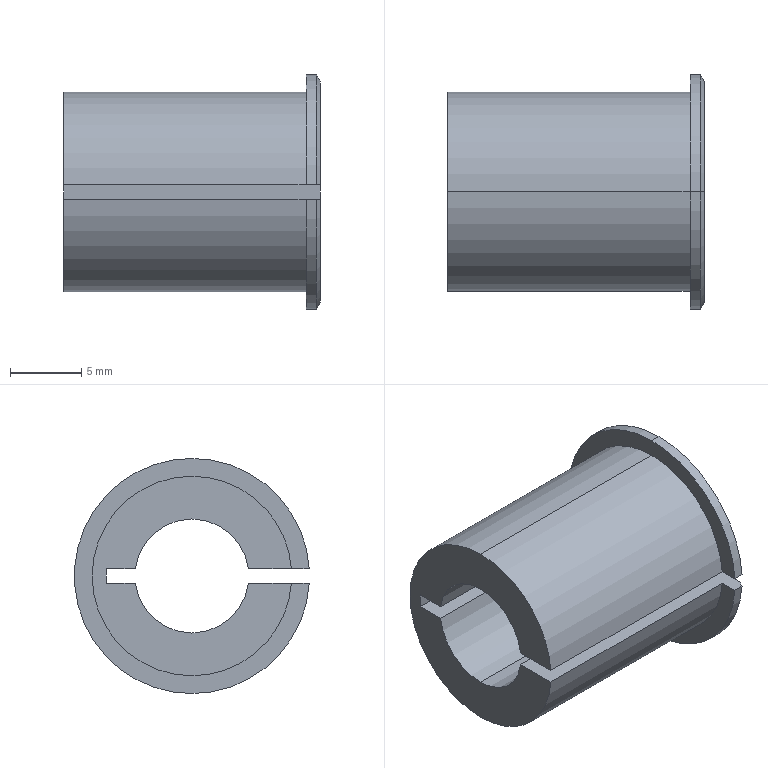Part | STEP file | _X2_8c0365745957_X0_14-8 | 1 solid | 20 faces | box 18 x 16.485 x 16.5 mm | volume 1831 mm3 | cylinder 9 | plane 8 | cone 3 | commonest cylinder face diameters 8 x3 14 x3 16.5 x3
STEP:
#1=CARTESIAN_POINT('',(21.547,-11.552,67.));
#2=VERTEX_POINT('',#1);
#3=CARTESIAN_POINT('',(21.547,-11.552,53.));
#4=VERTEX_POINT('',#3);
#5=CARTESIAN_POINT('',(21.547,-11.552,60.));
#6=DIRECTION('',(-1.,0.,0.));
#7=DIRECTION('',(0.,0.,1.));
#8=AXIS2_PLACEMENT_3D('',#5,#6,#7);
#9=CIRCLE('',#8,7.);
#10=EDGE_CURVE('',#2,#4,#9,.T.);
#11=ORIENTED_EDGE('',*,*,#10,.T.);
#12=CARTESIAN_POINT('',(4.547,-11.552,53.));
#13=VERTEX_POINT('',#12);
#14=CARTESIAN_POINT('',(21.547,-11.552,53.));
#15=DIRECTION('',(-1.,0.,0.));
#16=VECTOR('',#15,1000.);
#17=LINE('',#14,#16);
#18=EDGE_CURVE('',#4,#13,#17,.T.);
#19=ORIENTED_EDGE('',*,*,#18,.T.);
#20=CARTESIAN_POINT('',(4.547,-11.552,67.));
#21=VERTEX_POINT('',#20);
#22=CARTESIAN_POINT('',(4.547,-11.552,60.));
#23=DIRECTION('',(1.,0.,0.));
#24=DIRECTION('',(0.,0.,1.));
#25=AXIS2_PLACEMENT_3D('',#22,#23,#24);
#26=CIRCLE('',#25,7.);
#27=EDGE_CURVE('',#13,#21,#26,.T.);
#28=ORIENTED_EDGE('',*,*,#27,.T.);
#29=CARTESIAN_POINT('',(21.547,-11.552,67.));
#30=DIRECTION('',(-1.,0.,0.));
#31=VECTOR('',#30,1000.);
#32=LINE('',#29,#31);
#33=EDGE_CURVE('',#2,#21,#32,.T.);
#34=ORIENTED_EDGE('',*,*,#33,.F.);
#35=EDGE_LOOP('',(#11,#19,#28,#34));
#36=FACE_OUTER_BOUND('',#35,.T.);
#37=CARTESIAN_POINT('',(21.547,-11.552,60.));
#38=DIRECTION('',(-1.,0.,0.));
#39=DIRECTION('',(0.,0.,1.));
#40=AXIS2_PLACEMENT_3D('',#37,#38,#39);
#41=CYLINDRICAL_SURFACE('',#40,7.);
#42=ADVANCED_FACE('',(#36),#41,.T.);
#43=CARTESIAN_POINT('',(21.547,-18.534,60.5));
#44=VERTEX_POINT('',#43);
#45=CARTESIAN_POINT('',(21.547,-11.552,60.));
#46=DIRECTION('',(-1.,0.,0.));
#47=DIRECTION('',(0.,0.,1.));
#48=AXIS2_PLACEMENT_3D('',#45,#46,#47);
#49=CIRCLE('',#48,7.);
#50=EDGE_CURVE('',#44,#2,#49,.T.);
#51=ORIENTED_EDGE('',*,*,#50,.T.);
#52=ORIENTED_EDGE('',*,*,#33,.T.);
#53=CARTESIAN_POINT('',(4.547,-18.534,60.5));
#54=VERTEX_POINT('',#53);
#55=CARTESIAN_POINT('',(4.547,-11.552,60.));
#56=DIRECTION('',(1.,0.,0.));
#57=DIRECTION('',(0.,0.,1.));
#58=AXIS2_PLACEMENT_3D('',#55,#56,#57);
#59=CIRCLE('',#58,7.);
#60=EDGE_CURVE('',#21,#54,#59,.T.);
#61=ORIENTED_EDGE('',*,*,#60,.T.);
#62=CARTESIAN_POINT('',(21.547,-18.534,60.5));
#63=DIRECTION('',(1.,0.,0.));
#64=VECTOR('',#63,1000.);
#65=LINE('',#62,#64);
#66=EDGE_CURVE('',#54,#44,#65,.T.);
#67=ORIENTED_EDGE('',*,*,#66,.T.);
#68=EDGE_LOOP('',(#51,#52,#61,#67));
#69=FACE_OUTER_BOUND('',#68,.T.);
#70=CARTESIAN_POINT('',(21.547,-11.552,60.));
#71=DIRECTION('',(-1.,0.,0.));
#72=DIRECTION('',(0.,0.,1.));
#73=AXIS2_PLACEMENT_3D('',#70,#71,#72);
#74=CYLINDRICAL_SURFACE('',#73,7.);
#75=ADVANCED_FACE('',(#69),#74,.T.);
#76=CARTESIAN_POINT('',(4.547,-11.552,56.));
#77=VERTEX_POINT('',#76);
#78=CARTESIAN_POINT('',(4.547,-7.583,59.5));
#79=VERTEX_POINT('',#78);
#80=CARTESIAN_POINT('',(4.547,-11.552,60.));
#81=DIRECTION('',(1.,0.,0.));
#82=DIRECTION('',(0.,0.,-1.));
#83=AXIS2_PLACEMENT_3D('',#80,#81,#82);
#84=CIRCLE('',#83,4.);
#85=EDGE_CURVE('',#77,#79,#84,.T.);
#86=ORIENTED_EDGE('',*,*,#85,.F.);
#87=CARTESIAN_POINT('',(22.547,-11.552,56.));
#88=VERTEX_POINT('',#87);
#89=CARTESIAN_POINT('',(4.547,-11.552,56.));
#90=DIRECTION('',(1.,0.,0.));
#91=VECTOR('',#90,1000.);
#92=LINE('',#89,#91);
#93=EDGE_CURVE('',#77,#88,#92,.T.);
#94=ORIENTED_EDGE('',*,*,#93,.T.);
#95=CARTESIAN_POINT('',(22.547,-7.583,59.5));
#96=VERTEX_POINT('',#95);
#97=CARTESIAN_POINT('',(22.547,-11.552,60.));
#98=DIRECTION('',(-1.,0.,0.));
#99=DIRECTION('',(0.,0.,-1.));
#100=AXIS2_PLACEMENT_3D('',#97,#98,#99);
#101=CIRCLE('',#100,4.);
#102=EDGE_CURVE('',#96,#88,#101,.T.);
#103=ORIENTED_EDGE('',*,*,#102,.F.);
#104=CARTESIAN_POINT('',(4.547,-7.583,59.5));
#105=DIRECTION('',(1.,0.,0.));
#106=VECTOR('',#105,1000.);
#107=LINE('',#104,#106);
#108=EDGE_CURVE('',#79,#96,#107,.T.);
#109=ORIENTED_EDGE('',*,*,#108,.F.);
#110=EDGE_LOOP('',(#86,#94,#103,#109));
#111=FACE_OUTER_BOUND('',#110,.T.);
#112=CARTESIAN_POINT('',(4.547,-11.552,60.));
#113=DIRECTION('',(1.,0.,0.));
#114=DIRECTION('',(0.,0.,-1.));
#115=AXIS2_PLACEMENT_3D('',#112,#113,#114);
#116=CYLINDRICAL_SURFACE('',#115,4.);
#117=ADVANCED_FACE('',(#111),#116,.F.);
#118=CARTESIAN_POINT('',(21.547,-11.552,68.25));
#119=VERTEX_POINT('',#118);
#120=CARTESIAN_POINT('',(21.547,-11.552,51.75));
#121=VERTEX_POINT('',#120);
#122=CARTESIAN_POINT('',(21.547,-11.552,60.));
#123=DIRECTION('',(-1.,0.,0.));
#124=DIRECTION('',(0.,0.,-1.));
#125=AXIS2_PLACEMENT_3D('',#122,#123,#124);
#126=CIRCLE('',#125,8.25);
#127=EDGE_CURVE('',#119,#121,#126,.T.);
#128=ORIENTED_EDGE('',*,*,#127,.F.);
#129=CARTESIAN_POINT('',(22.258,-11.552,68.25));
#130=VERTEX_POINT('',#129);
#131=CARTESIAN_POINT('',(4.547,-11.552,68.25));
#132=DIRECTION('',(1.,0.,0.));
#133=VECTOR('',#132,1000.);
#134=LINE('',#131,#133);
#135=EDGE_CURVE('',#119,#130,#134,.T.);
#136=ORIENTED_EDGE('',*,*,#135,.T.);
#137=CARTESIAN_POINT('',(22.258,-11.552,51.75));
#138=VERTEX_POINT('',#137);
#139=CARTESIAN_POINT('',(22.258,-11.552,60.));
#140=DIRECTION('',(-1.,0.,0.));
#141=DIRECTION('',(0.,0.,-1.));
#142=AXIS2_PLACEMENT_3D('',#139,#140,#141);
#143=CIRCLE('',#142,8.25);
#144=EDGE_CURVE('',#130,#138,#143,.T.);
#145=ORIENTED_EDGE('',*,*,#144,.T.);
#146=CARTESIAN_POINT('',(4.547,-11.552,51.75));
#147=DIRECTION('',(1.,0.,0.));
#148=VECTOR('',#147,1000.);
#149=LINE('',#146,#148);
#150=EDGE_CURVE('',#121,#138,#149,.T.);
#151=ORIENTED_EDGE('',*,*,#150,.F.);
#152=EDGE_LOOP('',(#128,#136,#145,#151));
#153=FACE_OUTER_BOUND('',#152,.T.);
#154=CARTESIAN_POINT('',(4.547,-11.552,60.));
#155=DIRECTION('',(1.,0.,0.));
#156=DIRECTION('',(0.,0.,-1.));
#157=AXIS2_PLACEMENT_3D('',#154,#155,#156);
#158=CYLINDRICAL_SURFACE('',#157,8.25);
#159=ADVANCED_FACE('',(#153),#158,.T.);
#160=CARTESIAN_POINT('',(21.547,-19.787,59.5));
#161=VERTEX_POINT('',#160);
#162=CARTESIAN_POINT('',(21.547,-11.552,60.));
#163=DIRECTION('',(-1.,0.,0.));
#164=DIRECTION('',(0.,0.,-1.));
#165=AXIS2_PLACEMENT_3D('',#162,#163,#164);
#166=CIRCLE('',#165,8.25);
#167=EDGE_CURVE('',#121,#161,#166,.T.);
#168=ORIENTED_EDGE('',*,*,#167,.F.);
#169=ORIENTED_EDGE('',*,*,#150,.T.);
#170=CARTESIAN_POINT('',(22.258,-19.787,59.5));
#171=VERTEX_POINT('',#170);
#172=CARTESIAN_POINT('',(22.258,-11.552,60.));
#173=DIRECTION('',(-1.,0.,0.));
#174=DIRECTION('',(0.,0.,-1.));
#175=AXIS2_PLACEMENT_3D('',#172,#173,#174);
#176=CIRCLE('',#175,8.25);
#177=EDGE_CURVE('',#138,#171,#176,.T.);
#178=ORIENTED_EDGE('',*,*,#177,.T.);
#179=CARTESIAN_POINT('',(4.547,-19.787,59.5));
#180=DIRECTION('',(-1.,0.,0.));
#181=VECTOR('',#180,1000.);
#182=LINE('',#179,#181);
#183=EDGE_CURVE('',#171,#161,#182,.T.);
#184=ORIENTED_EDGE('',*,*,#183,.T.);
#185=EDGE_LOOP('',(#168,#169,#178,#184));
#186=FACE_OUTER_BOUND('',#185,.T.);
#187=CARTESIAN_POINT('',(4.547,-11.552,60.));
#188=DIRECTION('',(1.,0.,0.));
#189=DIRECTION('',(0.,0.,-1.));
#190=AXIS2_PLACEMENT_3D('',#187,#188,#189);
#191=CYLINDRICAL_SURFACE('',#190,8.25);
#192=ADVANCED_FACE('',(#186),#191,.T.);
#193=CARTESIAN_POINT('',(22.547,-11.552,67.75));
#194=VERTEX_POINT('',#193);
#195=CARTESIAN_POINT('',(22.547,-11.552,52.25));
#196=VERTEX_POINT('',#195);
#197=CARTESIAN_POINT('',(22.547,-11.552,60.));
#198=DIRECTION('',(-1.,0.,0.));
#199=DIRECTION('',(0.,0.,1.));
#200=AXIS2_PLACEMENT_3D('',#197,#198,#199);
#201=CIRCLE('',#200,7.75);
#202=EDGE_CURVE('',#194,#196,#201,.T.);
#203=ORIENTED_EDGE('',*,*,#202,.T.);
#204=CARTESIAN_POINT('',(22.258,-11.552,51.75));
#205=DIRECTION('',(-0.5,0.,-0.866));
#206=VECTOR('',#205,1000.);
#207=LINE('',#204,#206);
#208=EDGE_CURVE('',#196,#138,#207,.T.);
#209=ORIENTED_EDGE('',*,*,#208,.T.);
#210=ORIENTED_EDGE('',*,*,#144,.F.);
#211=CARTESIAN_POINT('',(22.258,-11.552,68.25));
#212=DIRECTION('',(-0.5,0.,0.866));
#213=VECTOR('',#212,1000.);
#214=LINE('',#211,#213);
#215=EDGE_CURVE('',#194,#130,#214,.T.);
#216=ORIENTED_EDGE('',*,*,#215,.F.);
#217=EDGE_LOOP('',(#203,#209,#210,#216));
#218=FACE_OUTER_BOUND('',#217,.T.);
#219=CARTESIAN_POINT('',(22.258,-11.552,60.));
#220=DIRECTION('',(-1.,0.,0.));
#221=DIRECTION('',(0.,0.,1.));
#222=AXIS2_PLACEMENT_3D('',#219,#220,#221);
#223=CONICAL_SURFACE('',#222,8.25,1.047);
#224=ADVANCED_FACE('',(#218),#223,.T.);
#225=CARTESIAN_POINT('',(22.547,-19.286,60.5));
#226=VERTEX_POINT('',#225);
#227=CARTESIAN_POINT('',(22.547,-11.552,60.));
#228=DIRECTION('',(-1.,0.,0.));
#229=DIRECTION('',(0.,0.,1.));
#230=AXIS2_PLACEMENT_3D('',#227,#228,#229);
#231=CIRCLE('',#230,7.75);
#232=EDGE_CURVE('',#226,#194,#231,.T.);
#233=ORIENTED_EDGE('',*,*,#232,.T.);
#234=ORIENTED_EDGE('',*,*,#215,.T.);
#235=CARTESIAN_POINT('',(22.258,-19.787,60.5));
#236=VERTEX_POINT('',#235);
#237=CARTESIAN_POINT('',(22.258,-11.552,60.));
#238=DIRECTION('',(-1.,0.,0.));
#239=DIRECTION('',(0.,0.,-1.));
#240=AXIS2_PLACEMENT_3D('',#237,#238,#239);
#241=CIRCLE('',#240,8.25);
#242=EDGE_CURVE('',#236,#130,#241,.T.);
#243=ORIENTED_EDGE('',*,*,#242,.F.);
#244=CARTESIAN_POINT('',(22.258,-19.787,60.5));
#245=CARTESIAN_POINT('',(22.354,-19.62,60.5));
#246=CARTESIAN_POINT('',(22.451,-19.453,60.5));
#247=CARTESIAN_POINT('',(22.547,-19.286,60.5));
#248=B_SPLINE_CURVE_WITH_KNOTS('',3,(#244,#245,#246,#247),.UNSPECIFIED.,.F.,.F.,(4,4),(0.,0.0005782),.UNSPECIFIED.);
#249=EDGE_CURVE('',#236,#226,#248,.T.);
#250=ORIENTED_EDGE('',*,*,#249,.T.);
#251=EDGE_LOOP('',(#233,#234,#243,#250));
#252=FACE_OUTER_BOUND('',#251,.T.);
#253=CARTESIAN_POINT('',(22.258,-11.552,60.));
#254=DIRECTION('',(-1.,0.,0.));
#255=DIRECTION('',(0.,0.,1.));
#256=AXIS2_PLACEMENT_3D('',#253,#254,#255);
#257=CONICAL_SURFACE('',#256,8.25,1.047);
#258=ADVANCED_FACE('',(#252),#257,.T.);
#259=ORIENTED_EDGE('',*,*,#18,.F.);
#260=CARTESIAN_POINT('',(21.547,-18.534,59.5));
#261=VERTEX_POINT('',#260);
#262=CARTESIAN_POINT('',(21.547,-11.552,60.));
#263=DIRECTION('',(-1.,0.,0.));
#264=DIRECTION('',(0.,0.,1.));
#265=AXIS2_PLACEMENT_3D('',#262,#263,#264);
#266=CIRCLE('',#265,7.);
#267=EDGE_CURVE('',#4,#261,#266,.T.);
#268=ORIENTED_EDGE('',*,*,#267,.T.);
#269=CARTESIAN_POINT('',(4.547,-18.534,59.5));
#270=VERTEX_POINT('',#269);
#271=CARTESIAN_POINT('',(21.547,-18.534,59.5));
#272=DIRECTION('',(-1.,0.,0.));
#273=VECTOR('',#272,1000.);
#274=LINE('',#271,#273);
#275=EDGE_CURVE('',#261,#270,#274,.T.);
#276=ORIENTED_EDGE('',*,*,#275,.T.);
#277=CARTESIAN_POINT('',(4.547,-11.552,60.));
#278=DIRECTION('',(1.,0.,0.));
#279=DIRECTION('',(0.,0.,1.));
#280=AXIS2_PLACEMENT_3D('',#277,#278,#279);
#281=CIRCLE('',#280,7.);
#282=EDGE_CURVE('',#270,#13,#281,.T.);
#283=ORIENTED_EDGE('',*,*,#282,.T.);
#284=EDGE_LOOP('',(#259,#268,#276,#283));
#285=FACE_OUTER_BOUND('',#284,.T.);
#286=CARTESIAN_POINT('',(21.547,-11.552,60.));
#287=DIRECTION('',(-1.,0.,0.));
#288=DIRECTION('',(0.,0.,1.));
#289=AXIS2_PLACEMENT_3D('',#286,#287,#288);
#290=CYLINDRICAL_SURFACE('',#289,7.);
#291=ADVANCED_FACE('',(#285),#290,.T.);
#292=CARTESIAN_POINT('',(4.547,-5.552,60.5));
#293=VERTEX_POINT('',#292);
#294=CARTESIAN_POINT('',(4.547,-7.583,60.5));
#295=VERTEX_POINT('',#294);
#296=CARTESIAN_POINT('',(4.547,-636.638,60.5));
#297=DIRECTION('',(0.,-1.,0.));
#298=VECTOR('',#297,1000.);
#299=LINE('',#296,#298);
#300=EDGE_CURVE('',#293,#295,#299,.T.);
#301=ORIENTED_EDGE('',*,*,#300,.T.);
#302=CARTESIAN_POINT('',(4.547,-15.52,60.5));
#303=VERTEX_POINT('',#302);
#304=CARTESIAN_POINT('',(4.547,-11.552,60.));
#305=DIRECTION('',(1.,0.,0.));
#306=DIRECTION('',(0.,0.,-1.));
#307=AXIS2_PLACEMENT_3D('',#304,#305,#306);
#308=CIRCLE('',#307,4.);
#309=EDGE_CURVE('',#295,#303,#308,.T.);
#310=ORIENTED_EDGE('',*,*,#309,.T.);
#311=CARTESIAN_POINT('',(4.547,-636.638,60.5));
#312=DIRECTION('',(0.,-1.,0.));
#313=VECTOR('',#312,1000.);
#314=LINE('',#311,#313);
#315=EDGE_CURVE('',#303,#54,#314,.T.);
#316=ORIENTED_EDGE('',*,*,#315,.T.);
#317=ORIENTED_EDGE('',*,*,#60,.F.);
#318=ORIENTED_EDGE('',*,*,#27,.F.);
#319=ORIENTED_EDGE('',*,*,#282,.F.);
#320=CARTESIAN_POINT('',(4.547,-15.52,59.5));
#321=VERTEX_POINT('',#320);
#322=CARTESIAN_POINT('',(4.547,-636.638,59.5));
#323=DIRECTION('',(0.,1.,0.));
#324=VECTOR('',#323,1000.);
#325=LINE('',#322,#324);
#326=EDGE_CURVE('',#270,#321,#325,.T.);
#327=ORIENTED_EDGE('',*,*,#326,.T.);
#328=CARTESIAN_POINT('',(4.547,-11.552,60.));
#329=DIRECTION('',(1.,0.,0.));
#330=DIRECTION('',(0.,0.,-1.));
#331=AXIS2_PLACEMENT_3D('',#328,#329,#330);
#332=CIRCLE('',#331,4.);
#333=EDGE_CURVE('',#321,#77,#332,.T.);
#334=ORIENTED_EDGE('',*,*,#333,.T.);
#335=ORIENTED_EDGE('',*,*,#85,.T.);
#336=CARTESIAN_POINT('',(4.547,-5.552,59.5));
#337=VERTEX_POINT('',#336);
#338=CARTESIAN_POINT('',(4.547,-636.638,59.5));
#339=DIRECTION('',(0.,1.,0.));
#340=VECTOR('',#339,1000.);
#341=LINE('',#338,#340);
#342=EDGE_CURVE('',#79,#337,#341,.T.);
#343=ORIENTED_EDGE('',*,*,#342,.T.);
#344=CARTESIAN_POINT('',(4.547,-5.552,-1434.79));
#345=DIRECTION('',(0.,0.,1.));
#346=VECTOR('',#345,1000.);
#347=LINE('',#344,#346);
#348=EDGE_CURVE('',#337,#293,#347,.T.);
#349=ORIENTED_EDGE('',*,*,#348,.T.);
#350=EDGE_LOOP('',(#301,#310,#316,#317,#318,#319,#327,#334,#335,#343,#349));
#351=FACE_OUTER_BOUND('',#350,.T.);
#352=CARTESIAN_POINT('',(4.547,-636.638,-1434.79));
#353=DIRECTION('',(-1.,0.,0.));
#354=DIRECTION('',(0.,0.,1.));
#355=AXIS2_PLACEMENT_3D('',#352,#353,#354);
#356=PLANE('',#355);
#357=ADVANCED_FACE('',(#351),#356,.T.);
#358=ORIENTED_EDGE('',*,*,#50,.F.);
#359=CARTESIAN_POINT('',(21.547,-19.787,60.5));
#360=VERTEX_POINT('',#359);
#361=CARTESIAN_POINT('',(21.547,-11.552,60.5));
#362=DIRECTION('',(0.,-1.,0.));
#363=VECTOR('',#362,1000.);
#364=LINE('',#361,#363);
#365=EDGE_CURVE('',#44,#360,#364,.T.);
#366=ORIENTED_EDGE('',*,*,#365,.T.);
#367=CARTESIAN_POINT('',(21.547,-11.552,60.));
#368=DIRECTION('',(-1.,0.,0.));
#369=DIRECTION('',(0.,0.,-1.));
#370=AXIS2_PLACEMENT_3D('',#367,#368,#369);
#371=CIRCLE('',#370,8.25);
#372=EDGE_CURVE('',#360,#119,#371,.T.);
#373=ORIENTED_EDGE('',*,*,#372,.T.);
#374=ORIENTED_EDGE('',*,*,#127,.T.);
#375=ORIENTED_EDGE('',*,*,#167,.T.);
#376=CARTESIAN_POINT('',(21.547,-11.552,59.5));
#377=DIRECTION('',(0.,1.,0.));
#378=VECTOR('',#377,1000.);
#379=LINE('',#376,#378);
#380=EDGE_CURVE('',#161,#261,#379,.T.);
#381=ORIENTED_EDGE('',*,*,#380,.T.);
#382=ORIENTED_EDGE('',*,*,#267,.F.);
#383=ORIENTED_EDGE('',*,*,#10,.F.);
#384=EDGE_LOOP('',(#358,#366,#373,#374,#375,#381,#382,#383));
#385=FACE_OUTER_BOUND('',#384,.T.);
#386=CARTESIAN_POINT('',(21.547,-11.552,60.));
#387=DIRECTION('',(-1.,0.,0.));
#388=DIRECTION('',(0.,0.,1.));
#389=AXIS2_PLACEMENT_3D('',#386,#387,#388);
#390=PLANE('',#389);
#391=ADVANCED_FACE('',(#385),#390,.T.);
#392=ORIENTED_EDGE('',*,*,#315,.F.);
#393=CARTESIAN_POINT('',(22.547,-15.52,60.5));
#394=VERTEX_POINT('',#393);
#395=CARTESIAN_POINT('',(4.547,-15.52,60.5));
#396=DIRECTION('',(1.,0.,0.));
#397=VECTOR('',#396,1000.);
#398=LINE('',#395,#397);
#399=EDGE_CURVE('',#303,#394,#398,.T.);
#400=ORIENTED_EDGE('',*,*,#399,.T.);
#401=CARTESIAN_POINT('',(22.547,-636.638,60.5));
#402=DIRECTION('',(0.,-1.,0.));
#403=VECTOR('',#402,1000.);
#404=LINE('',#401,#403);
#405=EDGE_CURVE('',#394,#226,#404,.T.);
#406=ORIENTED_EDGE('',*,*,#405,.T.);
#407=ORIENTED_EDGE('',*,*,#249,.F.);
#408=CARTESIAN_POINT('',(4.547,-19.787,60.5));
#409=DIRECTION('',(-1.,0.,0.));
#410=VECTOR('',#409,1000.);
#411=LINE('',#408,#410);
#412=EDGE_CURVE('',#236,#360,#411,.T.);
#413=ORIENTED_EDGE('',*,*,#412,.T.);
#414=ORIENTED_EDGE('',*,*,#365,.F.);
#415=ORIENTED_EDGE('',*,*,#66,.F.);
#416=EDGE_LOOP('',(#392,#400,#406,#407,#413,#414,#415));
#417=FACE_OUTER_BOUND('',#416,.T.);
#418=CARTESIAN_POINT('',(4.547,-636.638,60.5));
#419=DIRECTION('',(0.,0.,-1.));
#420=DIRECTION('',(-1.,0.,0.));
#421=AXIS2_PLACEMENT_3D('',#418,#419,#420);
#422=PLANE('',#421);
#423=ADVANCED_FACE('',(#417),#422,.T.);
#424=ORIENTED_EDGE('',*,*,#399,.F.);
#425=ORIENTED_EDGE('',*,*,#309,.F.);
#426=CARTESIAN_POINT('',(22.547,-7.583,60.5));
#427=VERTEX_POINT('',#426);
#428=CARTESIAN_POINT('',(4.547,-7.583,60.5));
#429=DIRECTION('',(-1.,0.,0.));
#430=VECTOR('',#429,1000.);
#431=LINE('',#428,#430);
#432=EDGE_CURVE('',#427,#295,#431,.T.);
#433=ORIENTED_EDGE('',*,*,#432,.F.);
#434=CARTESIAN_POINT('',(22.547,-11.552,60.));
#435=DIRECTION('',(-1.,0.,0.));
#436=DIRECTION('',(0.,0.,-1.));
#437=AXIS2_PLACEMENT_3D('',#434,#435,#436);
#438=CIRCLE('',#437,4.);
#439=EDGE_CURVE('',#394,#427,#438,.T.);
#440=ORIENTED_EDGE('',*,*,#439,.F.);
#441=EDGE_LOOP('',(#424,#425,#433,#440));
#442=FACE_OUTER_BOUND('',#441,.T.);
#443=CARTESIAN_POINT('',(4.547,-11.552,60.));
#444=DIRECTION('',(1.,0.,0.));
#445=DIRECTION('',(0.,0.,-1.));
#446=AXIS2_PLACEMENT_3D('',#443,#444,#445);
#447=CYLINDRICAL_SURFACE('',#446,4.);
#448=ADVANCED_FACE('',(#442),#447,.F.);
#449=ORIENTED_EDGE('',*,*,#432,.T.);
#450=ORIENTED_EDGE('',*,*,#300,.F.);
#451=CARTESIAN_POINT('',(22.547,-5.552,60.5));
#452=VERTEX_POINT('',#451);
#453=CARTESIAN_POINT('',(4.547,-5.552,60.5));
#454=DIRECTION('',(-1.,0.,0.));
#455=VECTOR('',#454,1000.);
#456=LINE('',#453,#455);
#457=EDGE_CURVE('',#452,#293,#456,.T.);
#458=ORIENTED_EDGE('',*,*,#457,.F.);
#459=CARTESIAN_POINT('',(22.547,-636.638,60.5));
#460=DIRECTION('',(0.,1.,0.));
#461=VECTOR('',#460,1000.);
#462=LINE('',#459,#461);
#463=EDGE_CURVE('',#427,#452,#462,.T.);
#464=ORIENTED_EDGE('',*,*,#463,.F.);
#465=EDGE_LOOP('',(#449,#450,#458,#464));
#466=FACE_OUTER_BOUND('',#465,.T.);
#467=CARTESIAN_POINT('',(4.547,-636.638,60.5));
#468=DIRECTION('',(0.,0.,1.));
#469=DIRECTION('',(1.,0.,0.));
#470=AXIS2_PLACEMENT_3D('',#467,#468,#469);
#471=PLANE('',#470);
#472=ADVANCED_FACE('',(#466),#471,.F.);
#473=ORIENTED_EDGE('',*,*,#342,.F.);
#474=ORIENTED_EDGE('',*,*,#108,.T.);
#475=CARTESIAN_POINT('',(22.547,-5.552,59.5));
#476=VERTEX_POINT('',#475);
#477=CARTESIAN_POINT('',(22.547,-636.638,59.5));
#478=DIRECTION('',(0.,1.,0.));
#479=VECTOR('',#478,1000.);
#480=LINE('',#477,#479);
#481=EDGE_CURVE('',#96,#476,#480,.T.);
#482=ORIENTED_EDGE('',*,*,#481,.T.);
#483=CARTESIAN_POINT('',(4.547,-5.552,59.5));
#484=DIRECTION('',(-1.,0.,0.));
#485=VECTOR('',#484,1000.);
#486=LINE('',#483,#485);
#487=EDGE_CURVE('',#476,#337,#486,.T.);
#488=ORIENTED_EDGE('',*,*,#487,.T.);
#489=EDGE_LOOP('',(#473,#474,#482,#488));
#490=FACE_OUTER_BOUND('',#489,.T.);
#491=CARTESIAN_POINT('',(4.547,-636.638,59.5));
#492=DIRECTION('',(0.,0.,1.));
#493=DIRECTION('',(1.,0.,0.));
#494=AXIS2_PLACEMENT_3D('',#491,#492,#493);
#495=PLANE('',#494);
#496=ADVANCED_FACE('',(#490),#495,.T.);
#497=ORIENTED_EDGE('',*,*,#93,.F.);
#498=ORIENTED_EDGE('',*,*,#333,.F.);
#499=CARTESIAN_POINT('',(22.547,-15.52,59.5));
#500=VERTEX_POINT('',#499);
#501=CARTESIAN_POINT('',(4.547,-15.52,59.5));
#502=DIRECTION('',(-1.,0.,0.));
#503=VECTOR('',#502,1000.);
#504=LINE('',#501,#503);
#505=EDGE_CURVE('',#500,#321,#504,.T.);
#506=ORIENTED_EDGE('',*,*,#505,.F.);
#507=CARTESIAN_POINT('',(22.547,-11.552,60.));
#508=DIRECTION('',(-1.,0.,0.));
#509=DIRECTION('',(0.,0.,-1.));
#510=AXIS2_PLACEMENT_3D('',#507,#508,#509);
#511=CIRCLE('',#510,4.);
#512=EDGE_CURVE('',#88,#500,#511,.T.);
#513=ORIENTED_EDGE('',*,*,#512,.F.);
#514=EDGE_LOOP('',(#497,#498,#506,#513));
#515=FACE_OUTER_BOUND('',#514,.T.);
#516=CARTESIAN_POINT('',(4.547,-11.552,60.));
#517=DIRECTION('',(1.,0.,0.));
#518=DIRECTION('',(0.,0.,-1.));
#519=AXIS2_PLACEMENT_3D('',#516,#517,#518);
#520=CYLINDRICAL_SURFACE('',#519,4.);
#521=ADVANCED_FACE('',(#515),#520,.F.);
#522=CARTESIAN_POINT('',(22.547,-19.286,59.5));
#523=VERTEX_POINT('',#522);
#524=CARTESIAN_POINT('',(22.547,-19.286,59.5));
#525=CARTESIAN_POINT('',(22.451,-19.453,59.5));
#526=CARTESIAN_POINT('',(22.354,-19.62,59.5));
#527=CARTESIAN_POINT('',(22.258,-19.787,59.5));
#528=B_SPLINE_CURVE_WITH_KNOTS('',3,(#524,#525,#526,#527),.UNSPECIFIED.,.F.,.F.,(4,4),(0.,0.0005782),.UNSPECIFIED.);
#529=EDGE_CURVE('',#523,#171,#528,.T.);
#530=ORIENTED_EDGE('',*,*,#529,.F.);
#531=CARTESIAN_POINT('',(22.547,-636.638,59.5));
#532=DIRECTION('',(0.,-1.,0.));
#533=VECTOR('',#532,1000.);
#534=LINE('',#531,#533);
#535=EDGE_CURVE('',#500,#523,#534,.T.);
#536=ORIENTED_EDGE('',*,*,#535,.F.);
#537=ORIENTED_EDGE('',*,*,#505,.T.);
#538=ORIENTED_EDGE('',*,*,#326,.F.);
#539=ORIENTED_EDGE('',*,*,#275,.F.);
#540=ORIENTED_EDGE('',*,*,#380,.F.);
#541=ORIENTED_EDGE('',*,*,#183,.F.);
#542=EDGE_LOOP('',(#530,#536,#537,#538,#539,#540,#541));
#543=FACE_OUTER_BOUND('',#542,.T.);
#544=CARTESIAN_POINT('',(4.547,-636.638,59.5));
#545=DIRECTION('',(0.,0.,-1.));
#546=DIRECTION('',(-1.,0.,0.));
#547=AXIS2_PLACEMENT_3D('',#544,#545,#546);
#548=PLANE('',#547);
#549=ADVANCED_FACE('',(#543),#548,.F.);
#550=ORIENTED_EDGE('',*,*,#135,.F.);
#551=ORIENTED_EDGE('',*,*,#372,.F.);
#552=ORIENTED_EDGE('',*,*,#412,.F.);
#553=ORIENTED_EDGE('',*,*,#242,.T.);
#554=EDGE_LOOP('',(#550,#551,#552,#553));
#555=FACE_OUTER_BOUND('',#554,.T.);
#556=CARTESIAN_POINT('',(4.547,-11.552,60.));
#557=DIRECTION('',(1.,0.,0.));
#558=DIRECTION('',(0.,0.,-1.));
#559=AXIS2_PLACEMENT_3D('',#556,#557,#558);
#560=CYLINDRICAL_SURFACE('',#559,8.25);
#561=ADVANCED_FACE('',(#555),#560,.T.);
#562=ORIENTED_EDGE('',*,*,#232,.F.);
#563=ORIENTED_EDGE('',*,*,#405,.F.);
#564=ORIENTED_EDGE('',*,*,#439,.T.);
#565=ORIENTED_EDGE('',*,*,#463,.T.);
#566=CARTESIAN_POINT('',(22.547,-5.552,-1434.79));
#567=DIRECTION('',(0.,0.,1.));
#568=VECTOR('',#567,1000.);
#569=LINE('',#566,#568);
#570=EDGE_CURVE('',#476,#452,#569,.T.);
#571=ORIENTED_EDGE('',*,*,#570,.F.);
#572=ORIENTED_EDGE('',*,*,#481,.F.);
#573=ORIENTED_EDGE('',*,*,#102,.T.);
#574=ORIENTED_EDGE('',*,*,#512,.T.);
#575=ORIENTED_EDGE('',*,*,#535,.T.);
#576=CARTESIAN_POINT('',(22.547,-11.552,60.));
#577=DIRECTION('',(-1.,0.,0.));
#578=DIRECTION('',(0.,0.,1.));
#579=AXIS2_PLACEMENT_3D('',#576,#577,#578);
#580=CIRCLE('',#579,7.75);
#581=EDGE_CURVE('',#196,#523,#580,.T.);
#582=ORIENTED_EDGE('',*,*,#581,.F.);
#583=ORIENTED_EDGE('',*,*,#202,.F.);
#584=EDGE_LOOP('',(#562,#563,#564,#565,#571,#572,#573,#574,#575,#582,#583));
#585=FACE_OUTER_BOUND('',#584,.T.);
#586=CARTESIAN_POINT('',(22.547,-636.638,-1434.79));
#587=DIRECTION('',(-1.,0.,0.));
#588=DIRECTION('',(0.,0.,1.));
#589=AXIS2_PLACEMENT_3D('',#586,#587,#588);
#590=PLANE('',#589);
#591=ADVANCED_FACE('',(#585),#590,.F.);
#592=ORIENTED_EDGE('',*,*,#457,.T.);
#593=ORIENTED_EDGE('',*,*,#348,.F.);
#594=ORIENTED_EDGE('',*,*,#487,.F.);
#595=ORIENTED_EDGE('',*,*,#570,.T.);
#596=EDGE_LOOP('',(#592,#593,#594,#595));
#597=FACE_OUTER_BOUND('',#596,.T.);
#598=CARTESIAN_POINT('',(4.547,-5.552,-1434.79));
#599=DIRECTION('',(0.,1.,0.));
#600=DIRECTION('',(0.,0.,1.));
#601=AXIS2_PLACEMENT_3D('',#598,#599,#600);
#602=PLANE('',#601);
#603=ADVANCED_FACE('',(#597),#602,.F.);
#604=ORIENTED_EDGE('',*,*,#208,.F.);
#605=ORIENTED_EDGE('',*,*,#581,.T.);
#606=ORIENTED_EDGE('',*,*,#529,.T.);
#607=ORIENTED_EDGE('',*,*,#177,.F.);
#608=EDGE_LOOP('',(#604,#605,#606,#607));
#609=FACE_OUTER_BOUND('',#608,.T.);
#610=CARTESIAN_POINT('',(22.258,-11.552,60.));
#611=DIRECTION('',(-1.,0.,0.));
#612=DIRECTION('',(0.,0.,1.));
#613=AXIS2_PLACEMENT_3D('',#610,#611,#612);
#614=CONICAL_SURFACE('',#613,8.25,1.047);
#615=ADVANCED_FACE('',(#609),#614,.T.);
#616=CLOSED_SHELL('',(#42,#75,#117,#159,#192,#224,#258,#291,#357,#391,#423,#448,#472,#496,#521,#549,#561,#591,#603,#615));
#617=MANIFOLD_SOLID_BREP('',#616);
#618=CARTESIAN_POINT('',(0.,0.,0.));
#619=DIRECTION('',(0.,0.,1.));
#620=DIRECTION('',(1.,0.,0.));
#621=AXIS2_PLACEMENT_3D('',#618,#619,#620);
#622=(LENGTH_UNIT()NAMED_UNIT(*)SI_UNIT(.MILLI.,.METRE.));
#623=UNCERTAINTY_MEASURE_WITH_UNIT(LENGTH_MEASURE(0.00001),#622,'','');
#624=(NAMED_UNIT(*)PLANE_ANGLE_UNIT()SI_UNIT($,.RADIAN.));
#625=(NAMED_UNIT(*)SI_UNIT($,.STERADIAN.)SOLID_ANGLE_UNIT());
#626=(GEOMETRIC_REPRESENTATION_CONTEXT(3)GLOBAL_UNCERTAINTY_ASSIGNED_CONTEXT((#623))GLOBAL_UNIT_ASSIGNED_CONTEXT((#622,#624,#625))REPRESENTATION_CONTEXT('',''));
#627=ADVANCED_BREP_SHAPE_REPRESENTATION('',(#617,#621),#626);